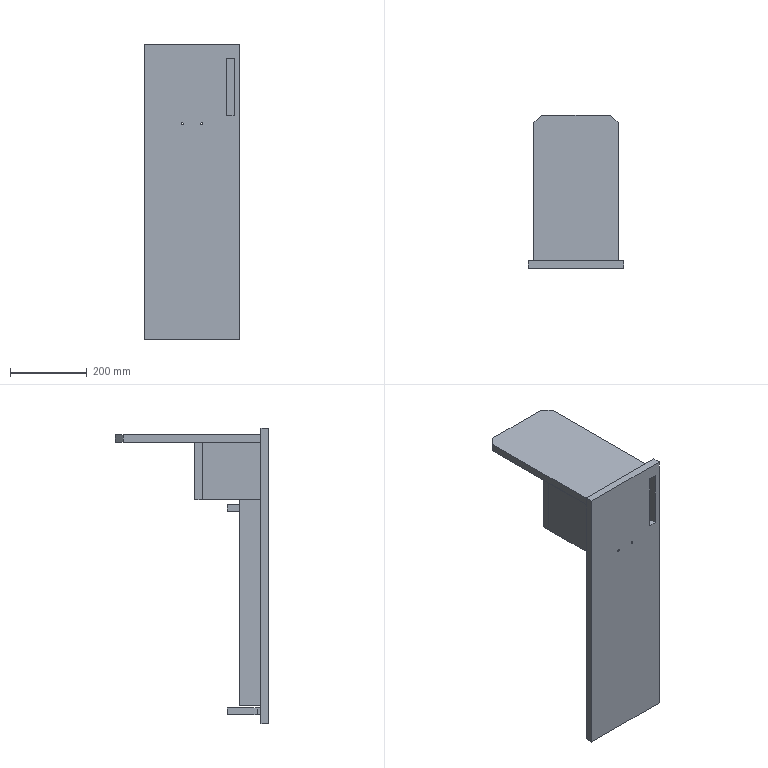Part | SolidWorks | features ICE 10, MoveFace 8, HoleWzd 2, MirrorSolid 2, Chamfer 1, Cut 1, DelFace 1, Extrusion 1, MoveCopyBody 1 | 11 solids | 126 faces | box 250 x 399.718 x 770 mm | volume 8667321 mm3 | plane 82 | cylinder 36 | cone 8 | commonest cylinder face diameters 5.5 x12 10 x8 35 x8 16 x4 37.8 x4